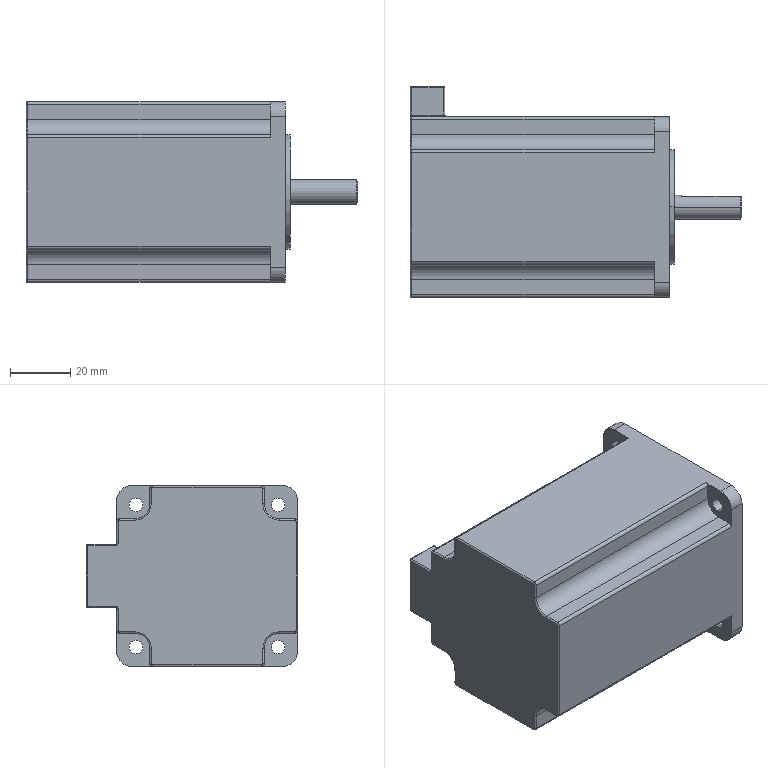Part | STEP file | 11-yk60hb86-04a11 | 1 solid | 136 faces | box 110 x 70 x 60 mm | volume 275885 mm3 | plane 61 | cylinder 52 | spline 20 | cone 3 | commonest cylinder face diameters 1 x24 2 x8 4.5 x8 10 x8 8 x2 38.1 x2